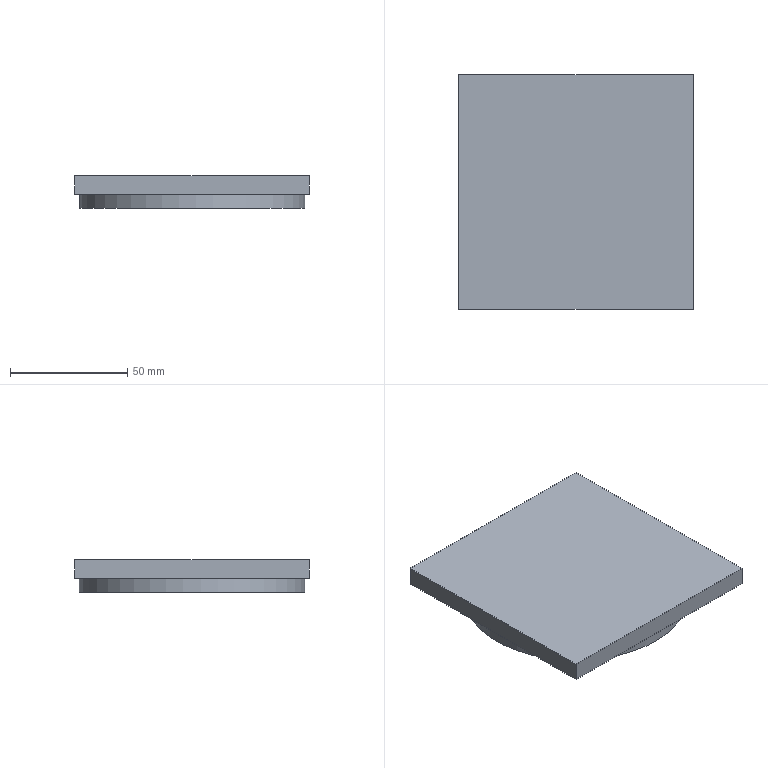NC program | NX | posted with a generic post | part box 100 x 100 x 14 mm
Lines 1 to 1665 of 1798, first 1410 of 1649 lines:
N10 G17 G21 G94 G90
(FLOOR_FACING , TOOL : FACEMILL-60)
N12 T01 M6
N14 G53
N16 G17 G0 G90 X-86. Y26. S4000 M3
N18 G43 Z50. H1
N20 Z3.
N22 G94 G1 Z0. F800.
N24 X-83.
N26 X83.
N28 X86.
N30 Z3.
N32 G0 Z50.
N34 X-86. Y-29.
N36 Z3.
N38 G1 Z0.
N40 X-83.
N42 X83.
N44 X86.
N46 Z3.
N48 G0 Z50.
N50 M5
(ADAPTIVE_MILLING , TOOL : D-12)
N52 T02 M6
N54 G53
N56 G17 G0 G90 X-65.089 Y0.29 S6000 M3
N58 G43 Z50. H2
N60 Z-4.
N62 G94 G1 X-64.939 Y0.301 Z-4.937 F4000.
N64 X-64.79 Y0.313 Z-5.308
N66 X-64.64 Y0.325 Z-5.58
N68 X-64.491 Y0.337 Z-5.8
N70 X-64.341 Y0.349 Z-5.984
N72 X-64.192 Y0.36 Z-6.142
N74 X-64.042 Y0.372 Z-6.28
N76 X-63.893 Y0.384 Z-6.4
N78 X-63.743 Y0.396 Z-6.505
N80 X-63.594 Y0.408 Z-6.598
N82 X-63.444 Y0.419 Z-6.679
N84 X-63.295 Y0.431 Z-6.75
N86 X-63.145 Y0.443 Z-6.81
N88 X-62.995 Y0.455 Z-6.862
N90 X-62.846 Y0.466 Z-6.905
N92 X-62.696 Y0.478 Z-6.939
N94 X-62.547 Y0.49 Z-6.966
N96 X-62.397 Y0.502 Z-6.985
N98 X-62.248 Y0.514 Z-6.996
N100 X-62.098 Y0.525 Z-7.
N102 X-60.075 Y0.685
N104 G3 X-59.097 Y1.329 R1.213
N106 X-58.517 Y3.223 R5.736
N108 X-58.075 Y9.387 R45.2
N110 X-58. Y23.273 R780.465
N112 G1 X-57.999 Y49.898
N114 G2 X-56.027 Y54.227 R6.381
N116 X-51.396 Y56.845 R10.806
N118 X-45.357 Y57.785 R27.098
N120 X-34.611 Y57.994 R195.318
N122 G1 X-27.736 Y58.
N124 X49.951 Y57.998
N126 G2 X54.264 Y55.988 R6.413
N128 X56.86 Y51.344 R10.871
N130 X57.795 Y45.178 R27.812
N132 X57.996 Y33.682 R218.985
N134 G1 X58. Y28.182
N136 X57.998 Y-49.951
N138 G2 X55.988 Y-54.264 R6.413
N140 X51.344 Y-56.858 R10.862
N142 X45.178 Y-57.795 R27.778
N144 X33.681 Y-57.996 R218.65
N146 G1 X28.181 Y-58.
N148 X-49.901 Y-57.999
N150 G2 X-54.229 Y-56.024 R6.379
N152 X-56.809 Y-51.512 R10.729
N154 X-57.768 Y-45.603 R26.178
N156 X-57.994 Y-34.607 R186.64
N158 G1 X-58. Y-27.732
N160 X-57.998 Y-2.557
N162 G2 X-57.555 Y2.538 R63.02
N164 G3 X-57.045 Y13.206 R117.899
N166 X-57. Y25.898 R812.081
N168 G1 X-56.999 Y46.573
N170 G2 X-53.638 Y53.302 R8.705
N172 X-48.111 Y55.912 R14.137
N174 X-41.055 Y56.815 R36.86
N176 X-27.932 Y56.997 R297.59
N178 G1 X-23.807 Y56.999
N180 X46.647 Y56.997
N182 G2 X53.27 Y53.673 R8.695
N184 X55.891 Y48.192 R13.997
N186 X56.804 Y41.263 R36.039
N188 X56.997 Y28.766 R269.693
N190 G1 X56.999 Y24.641
N192 X56.997 Y-46.647
N194 G2 X53.673 Y-53.269 R8.702
N196 X48.186 Y-55.891 R13.993
N198 X41.133 Y-56.811 R36.416
N200 X29.01 Y-56.996 R270.491
N202 G1 X23.51 Y-56.999
N204 X-46.647 Y-56.997
N206 G2 X-53.27 Y-53.673 R8.695
N208 X-55.891 Y-48.186 R13.977
N210 X-56.811 Y-41.133 R36.412
N212 X-56.997 Y-28.76 R275.722
N214 G1 X-56.999 Y-23.26
N216 Y-5.46
N218 G2 X-56.555 Y2.291 R94.488
N220 G3 X-56.023 Y17.178 R197.045
N222 G1 X-56.001 Y25.398
N224 X-55.999 Y43.698
N226 G2 X-51.39 Y52.531 R10.278
N228 X-45.402 Y54.982 R16.791
N230 X-37.833 Y55.829 R44.957
N232 X-23.085 Y55.998 R386.016
N234 G1 X43.465 Y55.999
N236 G2 X49.209 Y54.568 R10.642
N238 X53.648 Y49.437 R11.679
N240 X55.41 Y42.94 R22.137
N242 X55.939 Y34.086 R79.07
N244 X55.998 Y20.336 R815.92
N246 G1 X55.997 Y-43.714
N248 G2 X51.391 Y-52.528 R10.272
N250 X45.403 Y-54.98 R16.775
N252 X37.835 Y-55.829 R44.847
N254 X24.462 Y-55.997 R348.394
N256 G1 X20.337 Y-55.999
N258 X-43.713 Y-55.997
N260 G2 X-52.528 Y-51.39 R10.272
N262 X-54.98 Y-45.403 R16.777
N264 X-55.829 Y-37.835 R44.846
N266 X-55.997 Y-24.462 R348.85
N268 G1 X-55.999 Y-8.662
N270 G2 X-55.539 Y2.352 R136.996
N272 G3 X-55.014 Y20.041 R272.874
N274 G1 X-55.001 Y28.773
N276 X-55. Y40.948
N278 G2 X-54.278 Y45.868 R14.058
N280 X-49.275 Y51.756 R11.517
N282 X-42.963 Y54.049 R19.344
N284 X-34.761 Y54.852 R53.856
N286 X-19.387 Y54.998 R479.609
N288 G1 X40.522
N290 G2 X44.985 Y54.555 R16.446
N292 X51.595 Y49.534 R11.309
N294 X53.991 Y43.245 R18.746
N296 X54.841 Y35.048 R51.224
N298 X54.998 Y19.05 R468.312
N300 G1 Y-40.522
N302 G2 X54.555 Y-44.985 R16.442
N304 X49.533 Y-51.594 R11.306
N306 X43.246 Y-53.99 R18.772
N308 X35.423 Y-54.825 R49.898
N310 X21.925 Y-54.996 R358.645
N312 G1 X17.8 Y-54.998
N314 X-40.897
N316 G2 X-45.702 Y-54.335 R14.338
N318 X-51.791 Y-49.214 R11.487
N320 X-54.088 Y-42.755 R19.612
N322 X-54.868 Y-34.299 R56.752
N324 X-54.998 Y-19.175 R530.079
N326 X-54.949 Y-6.001 R682.38
N328 X-54.387 Y5.023 R474.825
N330 G3 X-54.005 Y24.528 R401.078
N332 G1 X-54.001 Y30.023
N334 G2 X-53.97 Y40.073 R507.626
N336 X-52.409 Y46.061 R12.952
N338 X-46.952 Y51.126 R12.89
N340 X-40.034 Y53.222 R22.867
N342 X-30.815 Y53.903 R72.319
N344 X-16.316 Y53.997 R728.258
N346 G1 X-3.103 Y53.998
N348 G2 X2.336 Y54.04 R52.026
N350 G3 X15.274 Y53.999 R846.67
N352 G1 X38.699 Y53.997
N354 G2 X43.528 Y53.458 R17.703
N356 X50.442 Y48.148 R12.015
N358 X52.93 Y41.633 R19.616
N360 X53.821 Y33.315 R52.129
N362 X53.995 Y19.567 R368.228
N364 G1 X53.998 Y2.94
N366 X54.077 Y1.572
N368 X54.013 Y-6.92
N370 X53.998 Y-11.398
N372 X53.997 Y-38.698
N374 G2 X53.457 Y-43.527 R17.702
N376 X48.148 Y-50.441 R12.014
N378 X41.634 Y-52.929 R19.612
N380 X33.191 Y-53.825 R52.556
N382 X19.817 Y-53.995 R367.411
N384 G1 X15.317 Y-53.998
N386 X2.888
N388 X1.771 Y-54.071
N390 G2 X-7.666 Y-54.01 R856.133
N392 G1 X-11.398 Y-53.999
N394 X-38.698 Y-53.997
N396 G2 X-43.527 Y-53.458 R17.701
N398 X-50.442 Y-48.147 R12.014
N400 X-52.929 Y-41.634 R19.611
N402 X-53.825 Y-33.19 R52.56
N404 X-53.995 Y-19.817 R367.553
N406 X-53.923 Y-6.143 R517.32
N408 G1 X-53.876 Y-4.74
N410 X-54.07 Y-1.81
N412 X-54.073 Y1.72
N414 X-53.845 Y5.246
N416 G3 X-53.129 Y14.406 R68.977
N418 X-53.001 Y36.073 R957.15
N420 G2 X-52.668 Y40.929 R25.722
N422 X-46.824 Y49.317 R12.573
N424 X-40.076 Y51.887 R20.428
N426 X-31.51 Y52.811 R53.827
N428 X-17.012 Y52.995 R377.523
N430 G1 X-10.689 Y53.004
N432 X-9.037 Y53.34
N434 X-5.538 Y53.816
N436 G2 X6.536 Y53.704 R56.591
N438 G3 X13.527 Y53.083 R43.417
N440 X26.148 Y52.999 R673.185
N442 G2 X38.073 Y52.967 R682.72
N444 X43.784 Y51.767 R14.82
N446 X49.812 Y45.976 R13.079
N448 X52.092 Y38.997 R22.642
N450 X52.873 Y29.788 R66.483
N452 X52.996 Y11.732 R709.652
N454 G1 X53.002 Y10.707
N456 X53.417 Y8.568
N458 X53.861 Y5.081
N460 X53.999 Y2.835
N462 G3 X55.868 Y1.914 R1.2
N464 X56.363 Y2.601 Z-6.964 R1.284
N466 G1 X56.883 Y4.008 Z-6.9
N468 X57.687 Y6.181 F15000.
N470 X57.741 Y6.386
N472 X57.761 Y6.597
N474 Y13.987
N476 G3 X56.945 Y28.72 R133.487
N478 G1 X55.966 Y37.534
N480 G3 X54.778 Y43.299 R31.882
N482 G1 X54.196 Y45.18
N484 G3 X51.934 Y49.405 R15.459
N486 G1 X50.831 Y50.793
N488 X49.715 Y52.17
N490 G3 X47.103 Y54.339 R8.82
N492 X44.86 Y55.321 R12.654
N494 X42.563 Y55.98 R21.548
N496 X39.835 Y56.326 R16.119
N498 X24.333 Y56.851 R857.968
N500 G1 X12.523 Y57.132
N502 G3 X12.062 Y57.051 R1.259
N504 G1 X9.867 Y56.202
N506 X8.438 Y55.644 Z-6.965 F4000.
N508 G3 X7.857 Y55.075 Z-7. R1.201
N510 X8.761 Y53.37 R1.2
N512 G1 X9.527 Y53.255
N514 G3 X13.501 Y52.453 R64.332
N516 X20.972 Y52.049 R67.24
N518 X35.148 Y51.991 R927.888
N520 G2 X40.475 Y51.396 R21.137
N522 X48.386 Y45.252 R13.159
N524 X50.925 Y38.222 R21.829
N526 X51.824 Y29.274 R59.201
N528 X51.993 Y14.99 R417.864
N530 G1 X52.009 Y14.837
N532 X52.748 Y12.019
N534 X53.01 Y10.669
N536 G3 X55.37 Y10.692 R1.2
N538 G1 X55.438 Y11.577 Z-6.962
N540 X55.491 Y12.464 Z-6.925
N542 X55.529 Y13.051 Z-6.9
N544 X55.67 Y15.276 F15000.
N546 Y28.577
N548 G3 X54.801 Y37.359 R44.796
N550 G1 X54.514 Y38.807
N552 X54.21 Y40.253
N554 G3 X52.016 Y46.039 R22.813
N556 X50.619 Y48.257 R26.338
N558 X48.528 Y50.989 R27.814
N560 X44.088 Y53.944 R11.075
N562 X41.594 Y54.75 R24.975
N564 X39.122 Y55.222 R20.211
N566 X34.715 Y55.59 R52.743
N568 G1 X16.468 Y56.341
N570 G3 X15.972 Y56.255 R1.243
N572 G1 X13.781 Y55.376
N574 X13.106 Y55.108 Z-6.931 F4000.
N576 X12.434 Y54.83 Z-6.962
N578 G3 X11.833 Y54.176 Z-7. R1.2
N580 X12.706 Y52.579 R1.2
N582 G1 X15.746 Y51.751
N584 G3 X21.132 Y51.166 R32.702
N586 X33.534 Y50.991 R358.026
N588 G2 X38.866 Y50.419 R23.067
N590 X47.299 Y43.995 R13.59
N592 X49.885 Y36.845 R22.44
N594 X50.817 Y27.651 R60.437
N596 X50.984 Y18.127 R338.825
N598 G1 X51.013 Y17.95
N600 G2 X52.015 Y14.814 R44.257
N602 G3 X54.202 Y14.498 R1.2
N604 X54.38 Y15.147 Z-6.971 R1.322
N606 G1 X54.497 Y16.826 Z-6.9
N608 X54.675 Y19.422 F15000.
N610 X54.679 Y22.271
N612 X54.664 Y25.121
N614 G3 X54.13 Y32.689 R71.988
N616 G1 X53.899 Y34.574
N618 X53.651 Y36.456
N620 G3 X52.248 Y41.973 R29.06
N622 X49.769 Y46.538 R18.664
N624 G1 X48.952 Y47.646
N626 X48.122 Y48.744
N628 G3 X44.773 Y51.675 R13.351
N630 X40.351 Y53.717 R18.733
N632 X37.11 Y54.31 R14.994
N634 G1 X19.254 Y55.574
N636 G3 X18.704 Y55.483 R1.222
N638 G1 X16.58 Y54.59
N640 X15.286 Y54.04 Z-6.96 F4000.
N642 G3 X14.675 Y53.336 Z-7. R1.2
N644 X15.492 Y51.812 R1.2
N646 G2 X17.881 Y51.029 R23.063
N648 G3 X22.767 Y50.272 R22.843
N650 X32.207 Y49.999 R188.287
N652 G2 X37.777 Y49.325 R23.278
N654 X46.191 Y42.819 R13.961
N656 X48.839 Y35.558 R22.833
N658 X49.799 Y26.367 R60.04
N660 G1 X49.946 Y20.837
N662 X49.997 Y20.593
N664 G2 X51.022 Y17.924 R31.153
N666 G3 X53.099 Y17.555 R1.2
N668 X53.366 Y18.329 Z-6.965 R1.291
N670 G1 X53.482 Y19.856 Z-6.9
N672 X53.682 Y22.531 F15000.
N674 X53.685 Y24.43
N676 X53.672 Y26.329
N678 G3 X53.196 Y31.358 R35.805
N680 G1 X52.346 Y36.461
N682 G3 X50.802 Y41.919 R25.345
N684 X49.361 Y44.722 R20.352
N686 G1 X48.671 Y45.844
N688 X47.969 Y46.959
N690 G3 X46.291 Y48.818 R9.254
N692 X43.876 Y50.501 R16.1
N694 X42.115 Y51.445 R23.694
N696 X39.157 Y52.509 R16.639
N698 X32.654 Y53.71 R40.631
N700 G1 X21.643 Y54.792
N702 G3 X21.04 Y54.695 R1.215
N704 G1 X18.99 Y53.787
N706 X17.728 Y53.223 Z-6.959 F4000.
N708 G3 X17.125 Y52.484 Z-7. R1.2
N710 X17.881 Y51.029 R1.2
N712 X20.706 Y50.021 R175.071
N714 X25.986 Y49.259 R26.266
N716 G1 X32.069 Y48.982
N718 G2 X38.049 Y47.789 R19.21
N720 X45.295 Y41.326 R14.502
N722 X47.878 Y33.891 R24.092
N724 X48.794 Y24.696 R62.398
N726 G1 X48.876 Y23.218
N728 G3 X49.421 Y22.01 R7.555
N730 G1 X50.033 Y20.504
N732 G3 X51.967 Y20.083 R1.2
N734 X52.35 Y20.964 Z-6.958 R1.265
N736 G1 X52.473 Y22.337 Z-6.9
N738 X52.698 Y24.858 F15000.
N740 X52.693 Y25.112
N742 X51.876 Y31.712
N744 G3 X50.249 Y38.883 R36.924
N746 G1 X49.938 Y39.812
N748 X49.617 Y40.738
N750 G3 X47.75 Y44.274 R15.825
N752 X46.562 Y45.893 R26.319
N754 X43.114 Y49.086 R16.268
N756 X41.574 Y50.09 R22.019
N758 X38.556 Y51.407 R14.583
N760 X34.245 Y52.396 R30.681
N762 G1 X23.77 Y54.015
N764 G3 X23.073 Y53.913 R1.209
N766 G1 X21.142 Y52.998
N768 X19.9 Y52.403 Z-6.958 F4000.
N770 G3 X19.315 Y51.643 Z-7. R1.2
N772 X20.008 Y50.252 R1.2
N774 X22.845 Y49.104 R29.665
N776 X27.716 Y48.321 R25.622
N778 G2 X33.01 Y47.807 R75.463
N780 X40.316 Y44.773 R15.451
N782 X45.305 Y37.949 R16.588
N784 X47.27 Y29.961 R31.219
N786 X47.699 Y25.607 R216.76
N788 G3 X47.887 Y25.172 R2.229
N790 G1 X48.978 Y22.923
N792 G3 X50.783 Y22.491 R1.2
N794 X51.263 Y23.436 Z-6.954 R1.258
N796 G1 X51.395 Y24.699 Z-6.9
N798 X51.655 Y27.17 F15000.
N800 X51.658 Y27.351
N802 X51.638 Y27.531
N804 X50.479 Y33.327
N806 G3 X48.535 Y39.57 R31.189
N808 X45.847 Y44.019 R20.503
N810 G1 X44.007 Y46.326
N812 X43.674 Y46.721
N814 X43.33 Y47.106
N816 G3 X42.421 Y47.844 R5.119
N818 G1 X41.532 Y48.409
N820 X40.635 Y48.963
N822 G3 X37.191 Y50.503 R17.436
N824 X32.493 Y51.608 R24.327
N826 G1 X31.793 Y51.684
N828 X31.092 Y51.742
N830 X26.592 Y52.03
N832 X23.931 Y51.797
N834 X22.371 Y51.655 Z-6.966 F4000.
N836 G3 X21.676 Y51.294 Z-7. R1.202
N838 X22.076 Y49.367 R1.2
N840 G2 X23.787 Y48.564 R19.134
N842 G3 X27.764 Y47.553 R16.138
N844 G2 X32.816 Y46.716 R66.271
N846 X43.365 Y38.67 R15.51
N848 X45.901 Y30.964 R25.883
N850 G1 X46.384 Y27.886
N852 X46.456 Y27.692
N854 X47.814 Y25.3
N856 G3 X49.494 Y24.875 R1.2
N858 X50.062 Y25.841 Z-6.951 R1.245
N860 G1 X50.222 Y27.031 Z-6.9
N862 X50.534 Y29.344 F15000.
N864 G3 X50.475 Y29.908 R1.221
N866 G1 X47.495 Y38.251
N868 G3 X45.291 Y42.404 R16.958
N870 X43.275 Y44.86 R28.269
N872 X38.235 Y48.591 R18.251
N874 X32.87 Y50.391 R20.252
N876 G1 X28.394 Y51.225
N878 X28.221 Y51.242
N880 X28.047 Y51.238
N882 X25.589 Y50.976
N884 X24.123 Y50.814 Z-6.962 F4000.
N886 G3 X23.379 Y50.367 Z-7. R1.2
N888 X23.787 Y48.564 R1.2
N890 X26.26 Y47.371 R27.438
N892 X30.47 Y46.245 R40.536
N894 G2 X36.285 Y44.008 R20.631
N896 X42.711 Y36.783 R16.598
N898 X44.753 Y30.503 R28.453
N900 G1 X44.886 Y30.154
N902 G2 X46.46 Y27.686 R37.891
N904 G3 X48.109 Y27.242 R1.2
N906 X48.706 Y28.2 Z-6.95 R1.244
N908 G1 X48.89 Y29.378 Z-6.9
N910 X49.232 Y31.571 F15000.
N912 G3 X49.12 Y32.293 R1.208
N914 G1 X46.146 Y38.242
N916 G3 X43.536 Y42.47 R27.585
N918 X40.353 Y45.612 R16.491
N920 X36.712 Y47.834 R21.93
N922 X32.402 Y49.603 R30.102
N924 G1 X30.178 Y50.32
N926 G3 X29.665 Y50.369 R1.231
N928 G1 X27.341 Y50.087
N930 X26.614 Y50.001 Z-6.931 F4000.
N932 X25.888 Y49.906 Z-6.962
N934 G3 X25.144 Y49.438 Z-7. R1.2
N936 X25.57 Y47.66 R1.2
N938 G2 X27.419 Y46.618 R42.594
N940 G3 X31.105 Y45.152 R44.01
N942 G2 X37.091 Y41.772 R20.158
N944 X42.226 Y34.442 R18.46
N946 G3 X42.772 Y33.086 R16.575
N948 G2 X44.907 Y30.122 R37.289
N950 G3 X46.987 Y30.252 R1.2
N952 X47.074 Y31.093 Z-6.964 R1.284
N954 G1 X46.826 Y32.575 Z-6.9
N956 X46.449 Y34.825 F15000.
N958 G3 X46.284 Y35.261 R1.26
N960 G1 X43.161 Y40.271
N962 G3 X39.246 Y44.64 R16.866
N964 X34.995 Y47.565 R33.497
N966 G1 X31.82 Y49.386
N968 G3 X31.019 Y49.528 R1.205
N970 G1 X28.916 Y49.165
N972 X27.547 Y48.924 Z-6.959 F4000.
N974 G3 X26.786 Y48.361 Z-7. R1.2
N976 X27.213 Y46.726 R1.2
N978 G2 X30.351 Y44.808 R103.908
N980 X34.751 Y42.049 R41.316
N982 X39.313 Y37.139 R19.154
N984 G1 X39.808 Y36.635
N986 X42.103 Y33.973
N988 X42.781 Y33.074
N990 G3 X44.788 Y33.215 R1.2
N992 X44.895 Y34.14 Z-6.96 R1.277
N994 G1 X44.628 Y35.525 Z-6.9
N996 X44.362 Y36.906 F15000.
N998 G3 X43.986 Y37.571 R1.206
N1000 G1 X34.067 Y46.488
N1002 G3 X33.528 Y46.767 R1.215
N1004 G1 X32.218 Y47.061
N1006 X30.435 Y47.457 Z-6.977 F4000.
N1008 G3 X29.903 Y47.424 Z-7. R1.212
N1010 X29.571 Y45.283 R1.2
N1012 G2 X39.36 Y37.092 R53.639
N1014 G3 X40.552 Y36.781 R1.201
N1016 G1 X40.702 Y36.824
N1018 X42.972 Y37.486 Z-6.9
N1020 X43.228 Y37.561 F15000.
N1022 X43.486 Y37.626
N1024 G2 X44.68 Y37.092 R1.201
N1026 G1 X46.419 Y34.405
N1028 X48.144 Y31.71
N1030 G2 X51.978 Y24.84 R83.783
N1032 X54.314 Y19.215 R48.636
N1034 X55.895 Y13.967 R67.704
N1036 X57.074 Y8.994 R85.182
N1038 X57.558 Y5.382 R31.681
N1040 G1 X57.827 Y1.819
N1042 G2 X57.285 Y0.723 R1.201
N1044 G1 X57.041 Y0.564
N1046 X55.059 Y-0.726 Z-7. F4000.
N1048 X54.765 Y-0.913
N1050 X54.481 Y-1.114
N1052 G3 X54.065 Y-1.943 R1.202
N1054 G1 X53.825 Y-5.45
N1056 G3 X53.203 Y-10.725 R73.541
N1058 X53.015 Y-18.922 R160.805
N1060 G1 X52.999 Y-26.398
N1062 G2 X52.967 Y-38.073 R664.405
N1064 X51.766 Y-43.784 R14.816
N1066 X45.977 Y-49.811 R13.082
N1068 X38.997 Y-52.091 R22.615
N1070 X29.788 Y-52.873 R66.443
N1072 X15.164 Y-52.998 R576.325
N1074 G1 X10.687 Y-53.005
N1076 X8.817 Y-53.377
N1078 X5.305 Y-53.839
N1080 X2.81 Y-54.003
N1082 G3 X1.885 Y-55.858 R1.2
N1084 X2.578 Y-56.365 Z-6.963 R1.282
N1086 G1 X3.973 Y-56.884 Z-6.9
N1088 X6.142 Y-57.69 F15000.
N1090 G3 X6.572 Y-57.765 R1.279
N1092 G1 X13.958 Y-57.688
N1094 G3 X28.689 Y-56.837 R156.463
N1096 G1 X37.511 Y-55.908
N1098 G3 X43.282 Y-54.749 R31.596
N1100 G1 X45.165 Y-54.175
N1102 G3 X49.395 Y-51.922 R15.326
N1104 G1 X50.783 Y-50.82
N1106 X52.16 Y-49.704
N1108 G3 X54.328 Y-47.091 R8.796
N1110 X55.308 Y-44.848 R12.641
N1112 X55.965 Y-42.55 R21.533
N1114 X56.308 Y-39.822 R16.108
N1116 G1 X56.482 Y-35.394
N1118 G3 X56.898 Y-22.104 R858.081
N1120 G1 X57.119 Y-12.696
N1122 G3 X57.035 Y-12.226 R1.254
N1124 G1 X56.163 Y-10.025
N1126 X55.615 Y-8.655 Z-6.962 F4000.
N1128 G3 X54.985 Y-8.058 Z-7. R1.2
N1130 X53.357 Y-8.934 R1.2
N1132 X52.466 Y-13.526 R100.643
N1134 X52.054 Y-20.73 R63.285
N1136 X51.989 Y-35.273 R972.405
N1138 G2 X51.396 Y-40.475 R20.763
N1140 X45.252 Y-48.386 R13.159
N1142 X38.221 Y-50.924 R21.858
N1144 X29.524 Y-51.813 R58.279
N1146 X14.992 Y-51.994 R397.837
N1148 G1 X14.793 Y-52.015
N1150 G2 X10.574 Y-53.027 R41.345
N1152 G3 X10.646 Y-55.393 R1.2
N1154 G1 X13.005 Y-55.549 Z-6.9
N1156 X15.182 Y-55.687 F15000.
N1158 X28.483
N1160 G3 X37.264 Y-54.818 R44.796
N1162 G1 X38.713 Y-54.531
N1164 X40.158 Y-54.227
N1166 G3 X45.944 Y-52.033 R22.813
N1168 X48.162 Y-50.637 R26.338
N1170 X50.895 Y-48.546 R27.858
N1172 X53.86 Y-44.11 R11.217
N1174 G1 X54.215 Y-43.143
N1176 X54.558 Y-42.172
N1178 G3 X55.238 Y-39.166 R17.69
N1180 X55.444 Y-36.97 R24.593
N1182 G1 X56.427 Y-16.142
N1184 G3 X56.337 Y-15.627 R1.229
N1186 G1 X55.444 Y-13.47
N1188 X54.9 Y-12.167 Z-6.96 F4000.
N1190 G3 X54.204 Y-11.554 Z-7. R1.2
N1192 X52.664 Y-12.38 R1.2
N1194 X51.666 Y-16.197 R81.779
N1196 X51.112 Y-22.556 R42.762
N1198 X50.98 Y-34.035 R700.701
N1200 G2 X50.216 Y-39.589 R20.192
N1202 X43.995 Y-47.299 R13.617
N1204 X36.842 Y-49.883 R22.414
N1206 X27.773 Y-50.812 R59.919
N1208 X18.15 Y-50.982 R315.35
N1210 G1 X17.909 Y-51.022
N1212 G2 X14.746 Y-52.027 R35.497
N1214 G3 X14.474 Y-54.235 R1.2
N1216 X15.087 Y-54.391 Z-6.973 R1.339
N1218 G1 X16.808 Y-54.512 Z-6.9
N1220 X19.354 Y-54.687 F15000.
N1222 X22.203 Y-54.691
N1224 X25.052 Y-54.676
N1226 G3 X32.621 Y-54.142 R71.988
N1228 G1 X34.506 Y-53.911
N1230 X36.388 Y-53.663
N1232 G3 X41.291 Y-52.478 R29.573
N1234 X43.747 Y-51.545 R21.871
N1236 X46.553 Y-49.91 R18.564
N1238 X50.309 Y-46.858 R33.876
N1240 X52.124 Y-44.476 R10.036
N1242 X53.137 Y-42.244 R14.319
N1244 X53.854 Y-39.964 R22.059
N1246 X54.279 Y-37.246 R16.511
N1248 G1 X55.548 Y-19.401
N1250 G3 X55.458 Y-18.853 R1.222
N1252 G1 X54.564 Y-16.714
N1254 X54.019 Y-15.422 Z-6.959 F4000.
N1256 G3 X53.313 Y-14.809 Z-7. R1.2
N1258 X51.786 Y-15.639 R1.2
N1260 X50.884 Y-18.402 R57.964
N1262 X50.201 Y-23.92 R30.084
N1264 X49.983 Y-32.707 R328.635
N1266 G2 X49.11 Y-38.496 R20.611
N1268 X42.819 Y-46.19 R13.987
N1270 X35.555 Y-48.837 R22.81
N1272 X26.24 Y-49.804 R60.605
N1274 G1 X20.835 Y-49.948
N1276 X20.585 Y-50.
N1278 G2 X17.882 Y-51.031 R24.663
N1280 G3 X17.518 Y-53.105 R1.2
N1282 X18.293 Y-53.373 Z-6.965 R1.29
N1284 G1 X19.818 Y-53.49 Z-6.9
N1286 X22.49 Y-53.691 F15000.
N1288 X24.389 Y-53.694
N1290 X26.288 Y-53.681
N1292 G3 X31.317 Y-53.205 R35.805
N1294 G1 X36.419 Y-52.355
N1296 G3 X41.878 Y-50.811 R25.345
N1298 X44.68 Y-49.37 R20.352
N1300 G1 X45.803 Y-48.681
N1302 X46.918 Y-47.978
N1304 G3 X48.777 Y-46.3 R9.254
N1306 X50.46 Y-43.885 R16.144
N1308 G1 X50.971 Y-42.986
N1310 X51.473 Y-42.083
N1312 G3 X52.721 Y-38.991 R16.215
N1314 X53.099 Y-37.068 R12.998
N1316 G1 X53.558 Y-33.217
N1318 X54.002 Y-29.364
N1320 X54.407 Y-25.516
N1322 X54.786 Y-21.666
N1324 G3 X54.69 Y-21.066 R1.215
N1326 G1 X53.785 Y-19.006
N1328 X53.224 Y-17.741 Z-6.959 F4000.
N1330 G3 X52.488 Y-17.136 Z-7. R1.2
N1332 X51.024 Y-17.904 R1.2
N1334 G2 X50.134 Y-20.309 R42.923
N1336 G3 X49.316 Y-25.187 R22.045
N1338 X48.982 Y-32.07 R318.188
N1340 G2 X47.788 Y-38.05 R19.215
N1342 X41.322 Y-45.295 R14.498
N1344 X33.885 Y-47.878 R24.091
N1346 X24.689 Y-48.795 R62.877
N1348 G3 X23.204 Y-48.882 R19.782
N1350 X22.338 Y-49.273 R4.503
N1352 G1 X20.49 Y-50.039
N1354 G3 X20.067 Y-51.96 R1.2
N1356 X20.955 Y-52.353 Z-6.958 R1.263
N1358 G1 X22.317 Y-52.475 Z-6.9
N1360 X24.842 Y-52.703 F15000.
N1362 X25.098 Y-52.699
N1364 X31.698 Y-51.881
N1366 G3 X38.868 Y-50.255 R36.924
N1368 G1 X39.798 Y-49.944
N1370 X40.724 Y-49.623
N1372 G3 X44.26 Y-47.756 R15.825
N1374 X45.879 Y-46.568 R26.319
N1376 X49.072 Y-43.119 R16.268
N1378 X50.076 Y-41.579 R21.998
N1380 X51.392 Y-38.561 R14.571
N1382 X52.381 Y-34.251 R30.689
N1384 G1 X53.995 Y-23.787
N1386 G3 X53.894 Y-23.093 R1.209
N1388 G1 X52.98 Y-21.151
N1390 X52.39 Y-19.907 Z-6.958 F4000.
N1392 G3 X51.631 Y-19.32 Z-7. R1.2
N1394 X50.232 Y-20.025 R1.2
N1396 X49.128 Y-22.786 R40.367
N1398 X48.322 Y-27.717 R24.908
N1400 G2 X47.807 Y-33.011 R75.55
N1402 X44.772 Y-40.317 R15.452
N1404 X37.949 Y-45.303 R16.6
N1406 X29.957 Y-47.269 R31.311
N1408 X25.666 Y-47.687 R145.988
N1410 G1 X25.411 Y-47.756
N1412 X22.945 Y-48.973
N1414 G3 X22.515 Y-50.768 R1.2
N1416 X23.464 Y-51.255 Z-6.953 R1.257
N1418 G1 X24.719 Y-51.388 Z-6.9
N1420 X27.191 Y-51.65 F15000.
N1422 X27.373 Y-51.654
N1424 X27.553 Y-51.633
N1426 X33.35 Y-50.474
N1428 G3 X39.592 Y-48.531 R31.189
N1430 X44.041 Y-45.843 R20.503
N1432 G1 X46.348 Y-44.002
N1434 X46.743 Y-43.67
N1436 X47.128 Y-43.326
N1438 G3 X47.865 Y-42.416 R5.09
N1440 G1 X48.429 Y-41.526
N1442 X48.982 Y-40.628
N1444 G3 X50.513 Y-37.181 R17.316
N1446 X51.597 Y-32.489 R24.17
N1448 G1 X51.67 Y-31.79
N1450 X51.725 Y-31.089
N1452 X51.984 Y-26.738
N1454 X51.751 Y-24.016
N1456 X51.615 Y-22.499 Z-6.964 F4000.
N1458 G3 X51.221 Y-21.776 Z-7. R1.201
N1460 X49.322 Y-22.218 R1.2
N1462 X48.339 Y-24.337 R27.149
N1464 X47.44 Y-28.514 R22.146
N1466 G2 X46.499 Y-33.663 R39.809
N1468 X38.889 Y-43.243 R15.396
N1470 X31.21 Y-45.854 R25.352
N1472 X27.923 Y-46.373 R417.82
N1474 G1 X27.669 Y-46.461
N1476 X25.402 Y-47.761
N1478 G3 X24.934 Y-49.502 R1.2
N1480 X25.896 Y-50.042 Z-6.952 R1.247
N1482 G1 X27.108 Y-50.191 Z-6.9
N1484 X29.459 Y-50.482 F15000.
N1486 G3 X30.01 Y-50.421 R1.223
N1488 G1 X38.353 Y-47.442
N1490 G3 X42.505 Y-45.237 R16.958
N1492 X44.961 Y-43.222 R28.027
N1494 X48.675 Y-38.171 R17.993
N1496 X50.434 Y-32.793 R20.049
N1498 G1 X51.21 Y-28.413
N1500 X51.226 Y-28.246
N1502 X51.222 Y-28.079
N1504 X50.965 Y-25.611
N1506 X50.806 Y-24.133 Z-6.963 F4000.
N1508 G3 X50.369 Y-23.394 Z-7. R1.2
N1510 X48.549 Y-23.805 R1.2
N1512 X47.309 Y-26.466 R27.632
N1514 X46.184 Y-30.719 R50.525
N1516 G2 X43.81 Y-36.606 R19.803
N1518 X36.669 Y-42.763 R16.688
N1520 X30.514 Y-44.75 R28.705
N1522 G1 X30.149 Y-44.886
N1524 G2 X27.607 Y-46.497 R25.703
N1526 G3 X27.936 Y-48.705 R1.2
N1528 X28.55 Y-48.692 Z-6.974 R1.38
N1530 G1 X30.263 Y-48.359 Z-6.9
N1532 X32.746 Y-47.874 F15000.
N1534 X34.087 Y-47.526
N1536 X35.425 Y-47.164
N1538 G3 X38.945 Y-45.634 R16.025
N1540 X42.607 Y-43.166 R35.401
N1542 G1 X43.583 Y-42.417
N1544 X44.543 Y-41.647
N1546 G3 X45.523 Y-40.688 R7.188
N1548 G1 X45.698 Y-40.452
N1550 X45.865 Y-40.211
N1552 X46.592 Y-39.074
N1554 X47.305 Y-37.93
N1556 G3 X49.265 Y-33.57 R21.279
N1558 G1 X50.373 Y-30.108
N1560 G3 X50.42 Y-29.586 R1.229
N1562 G1 X50.117 Y-27.271
N1564 X49.928 Y-25.872 Z-6.96 F4000.
N1566 G3 X49.416 Y-25.1 Z-7. R1.2
N1568 X47.713 Y-25.5 R1.2
N1570 X46.365 Y-27.959 R26.362
N1572 G1 X44.732 Y-32.15
N1574 G2 X35.243 Y-41.887 R17.723
N1576 G1 X33.157 Y-42.729
N1578 G2 X30.071 Y-44.938 R43.843
N1580 G3 X30.188 Y-47.002 R1.2
N1582 X31.047 Y-47.1 Z-6.963 R1.28
N1584 G1 X32.509 Y-46.857 Z-6.9
N1586 X34.772 Y-46.48 F15000.
N1588 G3 X35.21 Y-46.315 R1.259
N1590 G1 X40.22 Y-43.192
N1592 G3 X44.592 Y-39.279 R16.965
N1594 X47.527 Y-35.035 R33.778
N1596 G1 X49.374 Y-31.84
N1598 G3 X49.518 Y-31.038 R1.205
N1600 G1 X49.158 Y-28.931
N1602 X48.919 Y-27.558 Z-6.959 F4000.
N1604 G3 X48.361 Y-26.797 Z-7. R1.2
N1606 X46.714 Y-27.233 R1.2
N1608 G2 X45.102 Y-29.845 R33.751
N1610 X42.637 Y-33.934 R71.894
N1612 X37.186 Y-39.283 R19.273
N1614 X34.335 Y-41.808 R196.279
N1616 G1 X33.046 Y-42.798
N1618 G3 X33.177 Y-44.789 R1.2
N1620 X34.116 Y-44.906 Z-6.959 R1.267
N1622 G1 X35.486 Y-44.645 Z-6.9
N1624 X36.876 Y-44.379 F15000.
N1626 G3 X37.543 Y-44.003 R1.206
N1628 G1 X46.467 Y-34.081
N1630 G3 X46.746 Y-33.544 R1.216
N1632 G1 X47.036 Y-32.262
N1634 X47.443 Y-30.445 Z-6.979 F4000.
N1636 G3 X47.421 Y-29.947 Z-7. R1.218
N1638 X45.263 Y-29.585 R1.2
N1640 G1 X43.99 Y-31.491
N1642 X41.835 Y-34.302
N1644 X39.501 Y-36.966
N1646 X37.115 Y-39.354
N1648 G3 X36.811 Y-40.534 R1.201
N1650 G1 X36.853 Y-40.68
N1652 X37.507 Y-42.952 Z-6.9
N1654 X37.584 Y-43.216 F15000.
N1656 X37.65 Y-43.483
N1658 G2 X37.115 Y-44.674 R1.201
N1660 G1 X34.429 Y-46.413
N1662 X31.733 Y-48.138
N1664 G2 X24.864 Y-51.974 R83.994
N1666 X19.24 Y-54.313 R48.766
N1668 X12.82 Y-56.17 R61.026
N1670 X8.952 Y-56.869 R48.059
N1672 G1 X1.991 Y-57.833
N1674 G2 X0.806 Y-57.277 R1.201
N1676 G1 X0.659 Y-57.039
N1678 X-0.587 Y-55.029 Z-7. F4000.
N1680 X-0.75 Y-54.762
N1682 X-0.925 Y-54.504
N1684 G3 X-1.772 Y-54.071 R1.202
N1686 G1 X-5.306 Y-53.839
N1688 G3 X-10.842 Y-53.198 R79.259
N1690 X-21.531 Y-53.004 R211.753
N1692 G1 X-29.023 Y-52.999
N1694 G2 X-38.322 Y-52.957 R343.088
N1696 X-44.234 Y-51.55 R14.2
N1698 X-49.871 Y-45.867 R13.209
N1700 X-52.091 Y-38.997 R22.763
N1702 X-52.873 Y-29.788 R66.467
N1704 X-52.995 Y-10.736 R733.078
N1706 G1 X-53.374 Y-8.835
N1708 X-53.836 Y-5.334
N1710 X-53.878 Y-4.71
N1712 G3 X-55.704 Y-3.767 R1.2
N1714 X-56.239 Y-4.477 Z-6.962 R1.276
N1716 G1 X-56.745 Y-5.842 Z-6.9
N1718 X-57.565 Y-8.055 F15000.
N1720 X-57.62 Y-8.261
N1722 X-57.64 Y-8.472
N1724 Y-16.601
N1726 G3 X-56.566 Y-32.786 R122.501
N1728 G1 X-55.491 Y-40.843
N1730 G3 X-54.407 Y-44.813 R16.018
N1732 X-53.66 Y-46.417 R20.368
N1734 G1 X-53.022 Y-47.644
N1736 X-52.369 Y-48.863
N1738 G3 X-50.005 Y-51.879 R13.527
N1740 G1 X-49.383 Y-52.474
N1742 X-48.738 Y-53.043
N1744 G3 X-44.929 Y-55.224 R12.549
N1746 X-42.544 Y-55.916 R26.541
N1748 X-39.431 Y-56.342 R17.789
N1750 X-28.359 Y-56.762 R429.451
N1752 G1 X-12.58 Y-57.139
N1754 G3 X-12.109 Y-57.055 R1.254
N1756 G1 X-9.909 Y-56.184
N1758 X-8.537 Y-55.635 Z-6.963 F4000.
N1760 G3 X-7.941 Y-55.007 Z-7. R1.2
N1762 X-8.818 Y-53.377 R1.2
N1764 X-13.724 Y-52.441 R100.29
N1766 X-21.095 Y-52.049 R68.251
N1768 X-35.274 Y-51.989 R978.368
N1770 G2 X-40.475 Y-51.396 R20.764
N1772 X-48.386 Y-45.252 R13.158
N1774 X-50.924 Y-38.221 R21.86
N1776 X-51.814 Y-29.524 R58.305
N1778 X-52.003 Y-14.867 R439.529
N1780 G1 X-52.684 Y-12.299
N1782 X-53.001 Y-10.705
N1784 G3 X-55.364 Y-10.754 R1.2
N1786 G1 X-55.521 Y-13.113 Z-6.9
N1788 X-55.661 Y-15.312 F15000.
N1790 Y-28.614
N1792 G3 X-54.792 Y-37.395 R44.796
N1794 G1 X-54.505 Y-38.844
N1796 X-54.201 Y-40.289
N1798 G3 X-52.579 Y-44.949 R22.893
N1800 X-50.968 Y-47.654 R18.653
N1802 G1 X-48.958 Y-50.447
N1804 X-48.566 Y-50.952
N1806 X-48.156 Y-51.442
N1808 G3 X-47.273 Y-52.213 R5.492
N1810 X-45.839 Y-53.161 R19.04
N1812 X-44.065 Y-53.986 R11.432
N1814 X-41.572 Y-54.781 R21.782
N1816 X-39.094 Y-55.19 R17.118
N1818 X-30.258 Y-55.815 R178.675
N1820 G1 X-16.054 Y-56.447
N1822 G3 X-15.542 Y-56.358 R1.23
N1824 G1 X-13.382 Y-55.465
N1826 X-12.078 Y-54.921 Z-6.96 F4000.
N1828 G3 X-11.465 Y-54.227 Z-7. R1.2
N1830 X-12.292 Y-52.685 R1.2
N1832 X-16.315 Y-51.641 R76.545
N1834 X-22.555 Y-51.112 R43.81
N1836 X-34.035 Y-50.98 R704.313
N1838 G2 X-39.589 Y-50.216 R20.122
N1840 X-47.299 Y-43.995 R13.614
N1842 X-49.884 Y-36.842 R22.414
N1844 X-50.812 Y-27.773 R59.932
N1846 X-50.982 Y-18.15 R314.704
N1848 G1 X-51.022 Y-17.911
N1850 G2 X-52.028 Y-14.744 R35.667
N1852 G3 X-54.236 Y-14.471 R1.2
N1854 X-54.392 Y-15.085 Z-6.973 R1.339
N1856 G1 X-54.513 Y-16.806 Z-6.9
N1858 X-54.688 Y-19.351 F15000.
N1860 X-54.692 Y-22.201
N1862 X-54.677 Y-25.05
N1864 G3 X-54.143 Y-32.619 R71.988
N1866 G1 X-53.912 Y-34.503
N1868 X-53.664 Y-36.386
N1870 G3 X-52.478 Y-41.289 R29.573
N1872 X-51.546 Y-43.745 R21.871
N1874 X-49.911 Y-46.551 R18.564
N1876 X-46.859 Y-50.307 R33.875
N1878 X-44.477 Y-52.121 R10.029
N1880 X-42.244 Y-53.134 R14.307
N1882 X-39.964 Y-53.85 R22.055
N1884 X-37.246 Y-54.274 R16.508
N1886 G1 X-19.475 Y-55.53
N1888 G3 X-18.912 Y-55.434 R1.22
N1890 G1 X-16.823 Y-54.527
N1892 X-15.554 Y-53.971 Z-6.959 F4000.
N1894 G3 X-14.946 Y-53.239 Z-7. R1.2
N1896 X-15.713 Y-51.768 R1.2
N1898 X-18.741 Y-50.801 R32.742
N1900 X-24.624 Y-50.166 R35.442
N1902 X-32.957 Y-49.974 R610.638
N1904 G2 X-38.733 Y-49.03 R19.705
N1906 X-46.317 Y-42.604 R14.066
N1908 X-48.886 Y-35.31 R23.348
N1910 X-49.804 Y-26.24 R61.807
N1912 G1 X-49.948 Y-20.834
N1914 X-50. Y-20.585
N1916 G2 X-51.035 Y-17.87 R24.845
N1918 G3 X-53.109 Y-17.507 R1.2
N1920 X-53.377 Y-18.281 Z-6.965 R1.29
N1922 G1 X-53.494 Y-19.807 Z-6.9
N1924 X-53.696 Y-22.478 F15000.
N1926 X-53.698 Y-24.377
N1928 X-53.686 Y-26.276
N1930 G3 X-53.21 Y-31.305 R35.805
N1932 G1 X-52.359 Y-36.407
N1934 G3 X-50.816 Y-41.866 R25.345
N1936 X-49.375 Y-44.668 R20.352
N1938 G1 X-48.685 Y-45.791
N1940 X-47.983 Y-46.906
N1942 G3 X-46.304 Y-48.765 R9.254
N1944 X-43.889 Y-50.448 R16.133
N1946 G1 X-42.991 Y-50.959
N1948 X-42.087 Y-51.461
N1950 G3 X-38.995 Y-52.709 R16.208
N1952 X-37.072 Y-53.086 R13.006
N1954 G1 X-33.216 Y-53.545
N1956 X-29.359 Y-53.989
N1958 X-25.542 Y-54.391
N1960 X-21.724 Y-54.766
N1962 G3 X-21.124 Y-54.671 R1.215
N1964 G1 X-19.063 Y-53.766
N1966 X-17.798 Y-53.204 Z-6.959 F4000.
N1968 G3 X-17.193 Y-52.469 Z-7. R1.2
N1970 X-17.962 Y-51.004 R1.2
N1972 G2 X-20.238 Y-50.158 R32.513
N1974 G3 X-24.849 Y-49.343 R20.66
N1976 X-31.819 Y-48.997 R206.301
N1978 G2 X-37.816 Y-47.879 R19.921
N1980 X-45.294 Y-41.323 R14.472
N1982 X-47.878 Y-33.885 R24.092
N1984 X-48.795 Y-24.689 R62.879
N1986 G3 X-48.882 Y-23.204 R20.313
N1988 X-49.283 Y-22.317 R4.569
N1990 G1 X-50. Y-20.584
N1992 G3 X-51.922 Y-20.161 R1.2
N1994 X-52.314 Y-21.049 Z-6.958 R1.263
N1996 G1 X-52.437 Y-22.411 Z-6.9
N1998 X-52.664 Y-24.937 F15000.
N2000 X-52.66 Y-25.192
N2002 X-51.842 Y-31.792
N2004 G3 X-50.216 Y-38.963 R36.924
N2006 G1 X-49.905 Y-39.892
N2008 X-49.584 Y-40.819
N2010 G3 X-47.665 Y-44.428 R15.841
N2012 X-44.822 Y-47.809 R25.673
N2014 G1 X-44.264 Y-48.366
N2016 X-43.682 Y-48.898
N2018 G3 X-41.418 Y-50.326 R10.555
N2020 X-39.228 Y-51.196 R17.27
N2022 X-34.947 Y-52.306 R30.725
N2024 G1 X-34.22 Y-52.426
N2026 X-23.752 Y-54.008
N2028 G3 X-23.063 Y-53.908 R1.209
N2030 G1 X-21.117 Y-52.994
N2032 X-19.873 Y-52.404 Z-6.958 F4000.
N2034 G3 X-19.286 Y-51.646 Z-7. R1.2
N2036 X-19.99 Y-50.246 R1.2
N2038 G1 X-22.56 Y-49.196
N2040 G3 X-27.486 Y-48.341 R23.022
N2042 G2 X-32.887 Y-47.826 R88.583
N2044 X-40.018 Y-45. R15.638
N2046 X-45.207 Y-38.179 R16.372
N2048 X-47.203 Y-30.453 R30.191
N2050 X-47.687 Y-25.666 R105.838
N2052 G1 X-47.756 Y-25.415
N2054 X-48.972 Y-22.948
N2056 G3 X-50.767 Y-22.518 R1.2
N2058 X-51.253 Y-23.466 Z-6.953 R1.257
N2060 G1 X-51.386 Y-24.722 Z-6.9
N2062 X-51.648 Y-27.194 F15000.
N2064 X-51.652 Y-27.375
N2066 X-51.632 Y-27.556
N2068 X-50.472 Y-33.352
N2070 G3 X-48.529 Y-39.594 R31.189
N2072 X-45.841 Y-44.043 R20.503
N2074 G1 X-44.001 Y-46.351
N2076 X-43.668 Y-46.745
N2078 X-43.325 Y-47.131
N2080 G3 X-42.425 Y-47.884 R5.61
N2082 G1 X-41.71 Y-48.361
N2084 X-40.976 Y-48.81
N2086 G3 X-39.205 Y-49.652 R13.671
N2088 X-34.295 Y-51.203 R31.652
N2090 G1 X-26.101 Y-53.035
N2092 G3 X-25.294 Y-52.933 R1.205
N2094 G1 X-23.487 Y-52.011
N2096 X-22.259 Y-51.379 Z-6.958 F4000.
N2098 G3 X-21.698 Y-50.606 Z-7. R1.2
N2100 X-22.339 Y-49.273 R1.2
N2102 X-24.564 Y-48.26 R17.605
N2104 X-28.514 Y-47.439 R23.773
N2106 G2 X-33.662 Y-46.499 R39.807
N2108 X-43.243 Y-38.889 R15.395
N2110 X-45.854 Y-31.21 R25.351
N2112 X-46.374 Y-27.923 R431.371
N2114 G1 X-46.46 Y-27.671
N2116 X-47.777 Y-25.373
N2118 G3 X-49.518 Y-24.904 R1.2
N2120 X-50.058 Y-25.866 Z-6.952 R1.247
N2122 G1 X-50.207 Y-27.078 Z-6.9
N2124 X-50.498 Y-29.43 F15000.
N2126 G3 X-50.437 Y-29.98 R1.223
N2128 G1 X-47.457 Y-38.323
N2130 G3 X-45.253 Y-42.476 R16.958
N2132 X-43.237 Y-44.932 R28.096
N2134 X-38.189 Y-48.651 R18.066
N2136 X-32.816 Y-50.421 R20.1
N2138 G1 X-28.404 Y-51.214
N2140 X-28.236 Y-51.23
N2142 X-28.067 Y-51.226
N2144 X-25.601 Y-50.969
N2146 X-24.124 Y-50.81 Z-6.963 F4000.
N2148 G3 X-23.385 Y-50.373 Z-7. R1.2
N2150 X-23.796 Y-48.554 R1.2
N2152 X-26.522 Y-47.289 R26.446
N2154 X-30.717 Y-46.184 R52.05
N2156 G2 X-36.606 Y-43.81 R19.786
N2158 X-42.763 Y-36.669 R16.688
N2160 X-44.75 Y-30.514 R28.709
N2162 G1 X-44.885 Y-30.149
N2164 G2 X-46.519 Y-27.57 R30.467
N2166 G3 X-48.728 Y-27.901 R1.2
N2168 X-48.714 Y-28.512 Z-6.974 R1.381
N2170 G1 X-48.381 Y-30.227 Z-6.9
N2172 X-47.896 Y-32.709 F15000.
N2174 X-47.539 Y-34.087
N2176 X-47.166 Y-35.461
N2178 G3 X-43.257 Y-42.597 R19.313
N2180 X-41.82 Y-44.202 R31.205
N2182 X-36.138 Y-48.232 R19.983
N2184 X-33.592 Y-49.244 R21.008
N2186 G1 X-30.123 Y-50.365
N2188 G3 X-29.597 Y-50.413 R1.228
N2190 G1 X-27.286 Y-50.109
N2192 X-25.887 Y-49.92 Z-6.96 F4000.
N2194 G3 X-25.115 Y-49.407 Z-7. R1.2
N2196 X-25.515 Y-47.705 R1.2
N2198 X-27.957 Y-46.365 R25.88
N2200 G1 X-32.149 Y-44.732
N2202 G2 X-41.887 Y-35.243 R17.722
N2204 G1 X-42.729 Y-33.157
N2206 X-43.991 Y-31.49
N2208 X-44.893 Y-30.139
N2210 G3 X-46.959 Y-30.257 R1.2
N2212 X-47.056 Y-31.115 Z-6.963 R1.281
N2214 G1 X-46.812 Y-32.578 Z-6.9
N2216 X-46.435 Y-34.84 F15000.
N2218 G3 X-46.27 Y-35.278 R1.259
N2220 G1 X-43.147 Y-40.287
N2222 G3 X-39.231 Y-44.656 R16.813
N2224 X-34.977 Y-47.576 R33.588
N2226 G1 X-31.854 Y-49.365
N2228 G3 X-31.057 Y-49.507 R1.205
N2230 G1 X-28.947 Y-49.148
N2232 X-27.573 Y-48.91 Z-6.959 F4000.
N2234 G3 X-26.813 Y-48.352 Z-7. R1.2
N2236 X-27.247 Y-46.705 R1.2
N2238 G2 X-29.854 Y-45.095 R32.389
N2240 X-33.933 Y-42.637 R71.173
N2242 X-39.286 Y-37.181 R19.269
N2244 X-41.836 Y-34.301 R87.494
N2246 G1 X-42.824 Y-33.012
N2248 G3 X-44.818 Y-33.144 R1.2
N2250 X-44.933 Y-34.082 Z-6.959 R1.267
N2252 G1 X-44.671 Y-35.453 Z-6.9
N2254 X-44.404 Y-36.843 F15000.
N2256 G3 X-44.029 Y-37.508 R1.206
N2258 G1 X-34.118 Y-46.444
N2260 G3 X-33.579 Y-46.723 R1.215
N2262 G1 X-32.295 Y-47.013
N2264 X-30.481 Y-47.418 Z-6.979 F4000.
N2266 G3 X-29.98 Y-47.396 Z-7. R1.217
N2268 X-29.621 Y-45.239 R1.2
N2270 G1 X-31.526 Y-43.965
N2272 X-34.336 Y-41.807
N2274 X-36.998 Y-39.471
N2276 X-39.295 Y-37.172
N2278 G3 X-40.477 Y-36.867 R1.201
N2280 G1 X-40.628 Y-36.911
N2282 X-42.899 Y-37.567 Z-6.9
N2284 X-43.16 Y-37.643 F15000.
N2286 X-43.423 Y-37.709
N2288 G2 X-44.616 Y-37.172 R1.201
N2290 G1 X-48.611 Y-30.963
N2292 G2 X-52.008 Y-24.756 R51.279
N2294 X-54.519 Y-18.559 R63.947
N2296 X-56.702 Y-9.956 R60.24
N2298 X-57.147 Y-6.828 R55.788
N2300 X-57.793 Y0.525 R154.676
N2302 G1 X-58.097 Y5.313
N2304 G2 X-57.068 Y6.577 R1.2
N2306 G1 X-56.661 Y6.635
N2308 X-54.416 Y6.958 Z-6.996 F4000.
N2310 X-54.322 Y6.983 Z-7.
N2312 G3 X-53.489 Y7.973 R1.201
N2314 G1 X-53.388 Y8.748
N2316 G3 X-52.482 Y13.582 R91.767
N2318 X-52.062 Y21.48 R76.303
N2320 X-51.992 Y35.274 R901.255
N2322 G2 X-51.398 Y40.476 R20.774
N2324 X-45.252 Y48.388 R13.164
N2326 X-38.221 Y50.926 R21.833
N2328 X-29.274 Y51.824 R59.186
N2330 X-14.99 Y51.992 R412.211
N2332 G1 X-14.787 Y52.013
N2334 G2 X-10.661 Y53.01 R39.334
N2336 G3 X-10.724 Y55.373 R1.2
N2338 G1 X-13.083 Y55.53 Z-6.9
N2340 X-15.269 Y55.67 F15000.
N2342 X-28.57
N2344 G3 X-37.351 Y54.801 R44.796
N2346 G1 X-38.8 Y54.514
N2348 X-40.245 Y54.21
N2350 G3 X-46.031 Y52.016 R22.813
N2352 X-48.249 Y50.619 R26.338
N2354 X-50.982 Y48.528 R27.847
N2356 X-53.944 Y44.091 R11.194
N2358 X-54.747 Y41.599 R22.986
N2360 X-55.183 Y39.125 R18.103
N2362 X-55.702 Y32.502 R105.428
N2364 G1 X-56.466 Y15.975
N2366 G3 X-56.376 Y15.461 R1.229
N2368 G1 X-55.484 Y13.302
N2370 X-54.94 Y11.998 Z-6.96 F4000.
N2372 G3 X-54.246 Y11.385 Z-7. R1.2
N2374 X-52.703 Y12.213 R1.2
N2376 X-51.681 Y16.168 R79.96
N2378 X-51.129 Y22.444 R44.015
N2380 X-50.983 Y34.036 R614.939
N2382 G2 X-50.218 Y39.59 R20.134
N2384 X-43.99 Y47.305 R13.619
N2386 X-36.843 Y49.886 R22.451
N2388 X-27.649 Y50.817 R60.495
N2390 X-18.151 Y50.981 R318.153
N2392 G1 X-17.904 Y51.022
N2394 G2 X-14.7 Y52.037 R33.246
N2396 G3 X-14.452 Y54.255 R1.2
N2398 X-15.047 Y54.4 Z-6.974 R1.381
N2400 G1 X-16.789 Y54.523 Z-6.9
N2402 X-19.308 Y54.697 F15000.
N2404 X-22.157 Y54.701
N2406 X-25.006 Y54.686
N2408 G3 X-32.575 Y54.152 R71.988
N2410 G1 X-34.46 Y53.921
N2412 X-36.342 Y53.673
N2414 G3 X-41.245 Y52.488 R29.573
N2416 X-43.701 Y51.555 R21.871
N2418 X-46.507 Y49.92 R18.564
N2420 X-50.263 Y46.868 R33.883
N2422 X-52.079 Y44.487 R10.064
N2424 X-53.095 Y42.256 R14.368
N2426 X-53.816 Y39.977 R22.117
N2428 X-54.246 Y37.26 R16.556
N2430 G1 X-55.556 Y19.388
N2432 G3 X-55.46 Y18.822 R1.22
N2434 G1 X-54.554 Y16.734
N2436 X-53.998 Y15.465 Z-6.959 F4000.
N2438 G3 X-53.266 Y14.857 Z-7. R1.2
N2440 X-51.794 Y15.625 R1.2
N2442 X-50.832 Y18.64 R35.99
N2444 X-50.181 Y24.509 R34.921
N2446 X-49.988 Y32.711 R428.16
N2448 G2 X-49.15 Y38.38 R20.829
N2450 X-42.818 Y46.194 R13.977
N2452 X-35.802 Y48.789 R22.604
N2454 X-26.866 Y49.778 R57.333
N2456 X-20.834 Y49.947 R572.926
N2458 G1 X-20.586 Y50.
N2460 G2 X-17.827 Y51.048 R25.036
N2462 G3 X-17.459 Y53.113 R1.2
N2464 X-18.242 Y53.389 Z-6.964 R1.288
N2466 G1 X-19.757 Y53.506 Z-6.9
N2468 X-22.435 Y53.709 F15000.
N2470 X-24.334 Y53.711
N2472 X-26.233 Y53.699
N2474 G3 X-31.262 Y53.223 R35.805
N2476 G1 X-36.364 Y52.372
N2478 G3 X-41.823 Y50.829 R25.345
N2480 X-44.625 Y49.388 R20.352
N2482 G1 X-45.489 Y48.856
N2484 X-46.345 Y48.314
N2486 G3 X-49.198 Y45.752 R13.859
N2488 X-50.562 Y44.013 R19.541
N2490 X-52.402 Y40.021 R13.378
N2492 X-53.321 Y35.702 R30.174
N2494 G1 X-53.407 Y34.971
N2496 X-54.797 Y21.638
N2498 G3 X-54.702 Y21.03 R1.215
N2500 G1 X-53.797 Y18.975
N2502 X-53.235 Y17.709 Z-6.959 F4000.
N2504 G3 X-52.499 Y17.105 Z-7. R1.2
N2506 X-51.035 Y17.876 R1.2
N2508 G2 X-50.178 Y20.185 R32.494
N2510 G3 X-49.351 Y24.85 R20.744
N2512 X-49.001 Y31.821 R206.8
N2514 G2 X-47.882 Y37.818 R19.934
N2516 X-41.326 Y45.297 R14.467
N2518 X-33.891 Y47.879 R24.084
N2520 X-24.695 Y48.795 R62.645
N2522 G3 X-23.219 Y48.881 R22.988
N2524 X-22.504 Y49.197 R3.716
N2526 G1 X-20.543 Y50.018
N2528 G3 X-20.12 Y51.933 R1.2
N2530 X-21.011 Y52.33 Z-6.958 R1.262
N2532 G1 X-22.367 Y52.453 Z-6.9
N2534 X-24.895 Y52.682 F15000.
N2536 X-25.151 Y52.678
N2538 X-31.751 Y51.86
N2540 G3 X-38.922 Y50.234 R36.924
N2542 G1 X-39.851 Y49.923
N2544 X-40.777 Y49.602
N2546 G3 X-44.313 Y47.735 R15.825
N2548 X-45.932 Y46.547 R26.319
N2550 X-49.651 Y42.27 R16.126
N2552 X-50.522 Y40.512 R14.21
N2554 X-51.746 Y37.049 R27.104
N2556 X-52.302 Y34.535 R35.23
N2558 G1 X-52.599 Y32.904
N2560 X-52.869 Y31.268
N2562 X-54.046 Y23.658
N2564 G3 X-53.946 Y22.965 R1.209
N2566 G1 X-53.032 Y21.02
N2568 X-52.442 Y19.776 Z-6.958 F4000.
N2570 G3 X-51.684 Y19.189 Z-7. R1.2
N2572 X-50.283 Y19.896 R1.2
N2574 X-49.155 Y22.714 R50.628
N2576 X-48.34 Y27.608 R24.295
N2578 G2 X-47.831 Y32.893 R86.013
N2580 X-44.926 Y40.122 R15.587
N2582 X-38.178 Y45.211 R16.386
N2584 X-30.451 Y47.206 R30.106
N2586 X-25.667 Y47.686 R101.041
N2588 G1 X-25.391 Y47.761
N2590 X-22.929 Y48.986
N2592 G3 X-22.5 Y50.775 R1.2
N2594 X-23.45 Y51.265 Z-6.953 R1.257
N2596 G1 X-24.702 Y51.399 Z-6.9
N2598 X-27.174 Y51.663 F15000.
N2600 X-27.356 Y51.666
N2602 X-27.537 Y51.646
N2604 X-33.334 Y50.487
N2606 G3 X-39.576 Y48.543 R31.189
N2608 X-44.025 Y45.855 R20.503
N2610 G1 X-46.332 Y44.015
N2612 X-46.727 Y43.682
N2614 X-47.112 Y43.339
N2616 G3 X-47.849 Y42.429 R5.097
N2618 G1 X-48.414 Y41.539
N2620 X-48.967 Y40.641
N2622 G3 X-50.499 Y37.195 R17.343
N2624 X-51.589 Y32.501 R24.205
N2626 G1 X-51.662 Y31.802
N2628 X-51.718 Y31.101
N2630 X-51.981 Y26.75
N2632 X-51.726 Y24.061
N2634 X-51.578 Y22.573 Z-6.963 F4000.
N2636 G3 X-51.155 Y21.836 Z-7. R1.2
N2638 X-49.319 Y22.237 R1.2
N2640 X-48.266 Y24.55 R18.639
N2642 X-47.376 Y28.997 R26.721
N2644 G2 X-46.287 Y34.382 R31.175
N2646 X-38.936 Y43.221 R15.368
N2648 X-31.405 Y45.82 R25.088
N2650 X-27.92 Y46.374 R164.49
N2652 G1 X-27.66 Y46.464
N2654 G2 X-25.33 Y47.791 R41.688
N2656 G3 X-24.876 Y49.546 R1.2
N2658 X-25.828 Y50.071 Z-6.952 R1.254
N2660 G1 X-27.058 Y50.223 Z-6.9
N2662 X-29.386 Y50.512 F15000.
N2664 G3 X-29.938 Y50.452 R1.223
N2666 G1 X-38.281 Y47.472
N2668 G3 X-42.433 Y45.268 R16.958
N2670 X-44.889 Y43.252 R28.175
N2672 X-48.614 Y38.208 R18.15
N2674 X-50.399 Y32.838 R20.198
N2676 G1 X-51.208 Y28.415
N2678 X-51.225 Y28.246
N2680 X-51.221 Y28.075
N2682 X-50.964 Y25.613
N2684 X-50.805 Y24.134 Z-6.963 F4000.
N2686 G3 X-50.37 Y23.396 Z-7. R1.2
N2688 X-48.548 Y23.808 R1.2
N2690 X-47.351 Y26.358 R32.259
N2692 X-46.309 Y30.234 R38.678
N2694 G2 X-44.2 Y35.962 R21.663
N2696 X-37.006 Y42.603 R16.476
N2698 X-30.512 Y44.752 R27.976
N2700 G1 X-30.143 Y44.89
N2702 G2 X-27.638 Y46.477 R25.272
N2704 G3 X-27.201 Y48.113 R1.2
N2706 X-28.17 Y48.718 Z-6.95 R1.25
N2708 G1 X-29.333 Y48.902 Z-6.9
N2710 X-31.521 Y49.249 F15000.
N2712 G3 X-32.245 Y49.137 R1.207
N2714 G1 X-38.194 Y46.163
N2716 G3 X-42.484 Y43.505 R27.338
N2718 X-45.572 Y40.376 R16.71
N2720 X-47.768 Y36.835 R21.518
N2722 X-49.654 Y32.337 R31.842
N2724 G1 X-50.423 Y30.015
N2726 G3 X-50.474 Y29.48 R1.226
N2728 G1 X-50.169 Y27.176
N2730 X-49.979 Y25.776 Z-6.96 F4000.
N2732 G3 X-49.466 Y25.005 Z-7. R1.2
N2734 X-47.763 Y25.407 R1.2
N2736 X-46.369 Y27.953 R27.904
N2738 G1 X-44.736 Y32.148
N2740 G2 X-35.248 Y41.888 R17.708
N2742 G1 X-33.158 Y42.73
N2744 X-31.648 Y43.877
N2746 X-30.093 Y44.924
N2748 G3 X-30.206 Y46.982 R1.2
N2750 X-31.071 Y47.084 Z-6.962 R1.279
N2752 G1 X-32.526 Y46.843 Z-6.9
N2754 X-34.794 Y46.466 F15000.
N2756 G3 X-35.232 Y46.301 R1.259
N2758 G1 X-40.242 Y43.177
N2760 G3 X-44.612 Y39.264 R16.912
N2762 X-47.543 Y35.017 R33.768
N2764 G1 X-49.364 Y31.857
N2766 G3 X-49.508 Y31.057 R1.205
N2768 G1 X-49.149 Y28.948
N2770 X-48.911 Y27.574 Z-6.959 F4000.
N2772 G3 X-48.354 Y26.813 Z-7. R1.2
N2774 X-46.704 Y27.25 R1.2
N2776 G2 X-45.095 Y29.854 R33.097
N2778 X-42.649 Y33.921 R70.88
N2780 X-37.195 Y39.279 R19.169
N2782 G1 X-34.444 Y41.719
N2784 X-32.96 Y42.864
N2786 G3 X-33.089 Y44.851 R1.2
N2788 X-34.032 Y44.971 Z-6.959 R1.266
N2790 G1 X-35.397 Y44.71 Z-6.9
N2792 X-36.791 Y44.444 F15000.
N2794 G3 X-37.456 Y44.069 R1.206
N2796 G1 X-46.447 Y34.111
N2798 G3 X-46.727 Y33.572 R1.215
N2800 G1 X-47.015 Y32.295
N2802 X-47.423 Y30.473 Z-6.979 F4000.
N2804 G3 X-47.403 Y29.98 Z-7. R1.219
N2806 X-45.242 Y29.614 R1.2
N2808 G1 X-44.048 Y31.41
N2810 X-41.905 Y34.217
N2812 X-39.583 Y36.878
N2814 X-37.115 Y39.36
N2816 G3 X-36.954 Y40.869 R1.212
N2818 G1 X-38.01 Y42.514
N2820 X-38.091 Y42.64 Z-6.996
N2822 X-38.172 Y42.767 Z-6.985
N2824 X-38.253 Y42.893 Z-6.966